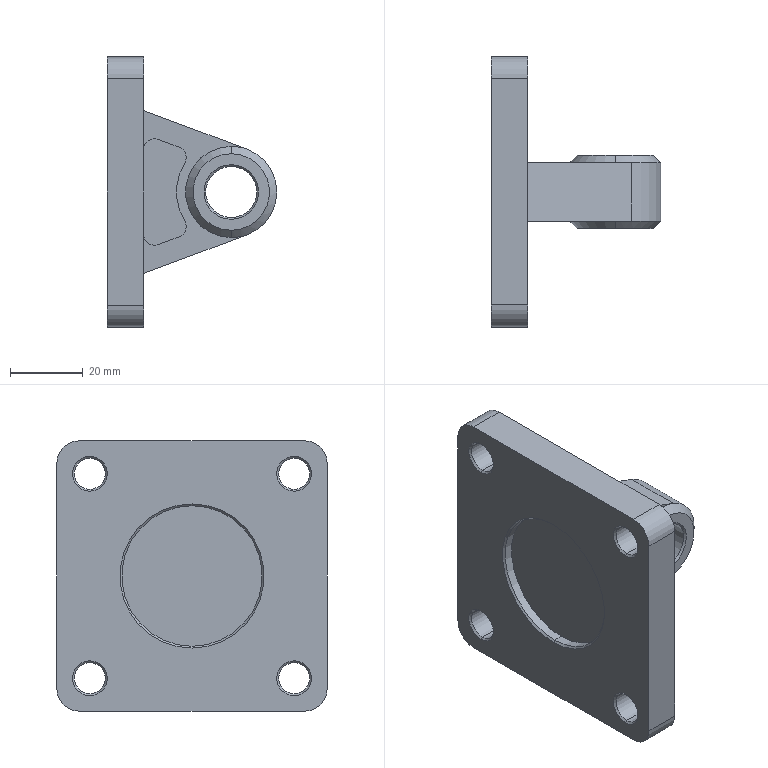Part | STEP file | F_SC63CA_F-SC63CA | 1 solid | 94 faces | box 46.5 x 74 x 74 mm | volume 62495 mm3 | cylinder 37 | cone 34 | plane 23 | commonest cylinder face diameters 6 x10 8.5 x8 13.5 x8 12 x4 14 x2 30 x2